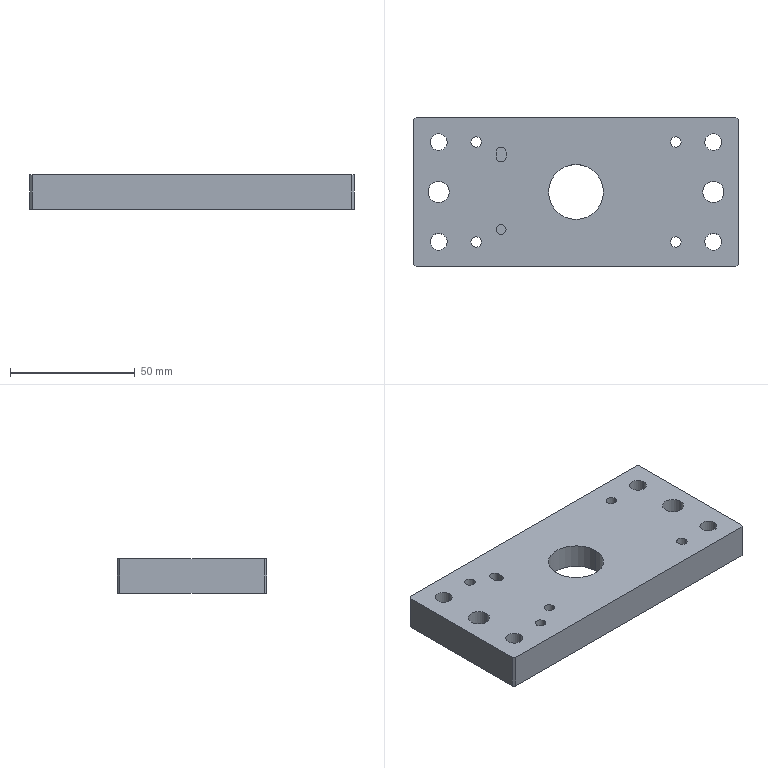Part | STEP file | PN_0013 Plate 3_Default | 1 solid | 43 faces | box 130 x 60 x 14 mm | volume 92668 mm3 | cylinder 28 | plane 15 | commonest cylinder face diameters 4.2 x8 6.8 x8 4 x4 8.5 x4 22 x2 51 x2